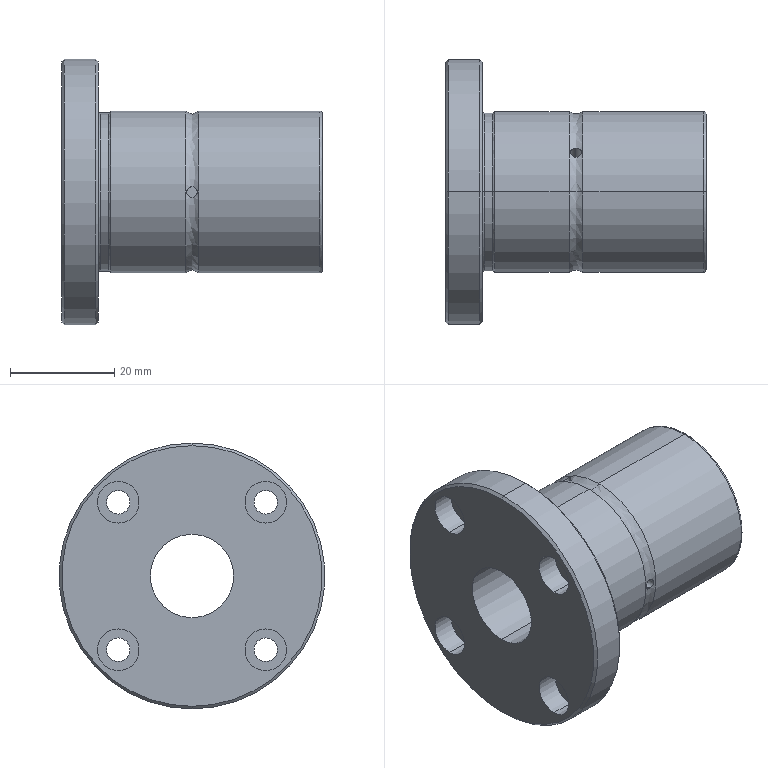Part | STEP file | SceondHI_LF 16 FTLF Cylindar_Default | 1 solid | 51 faces | box 50 x 51 x 51 mm | volume 35392 mm3 | cylinder 32 | spline 8 | plane 7 | cone 4 | commonest cylinder face diameters 4.5 x8 8 x8 2 x6 31 x4 16 x2 30.4 x2